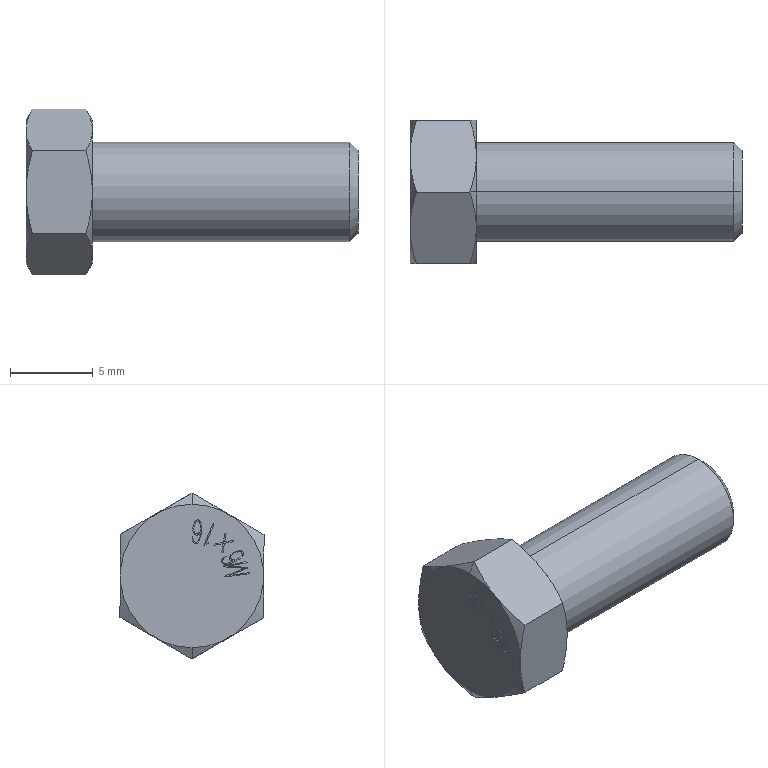Part | SolidWorks | features ICE 2, Chamfer 1, Extrusion 1, MirrorPattern 1, RevCut 1 | 1 solid | 98 faces | box 20 x 8.68 x 10 mm | volume 708.376 mm3 | plane 58 | spline 32 | cone 6 | cylinder 2 | commonest cylinder face diameters 6 x2